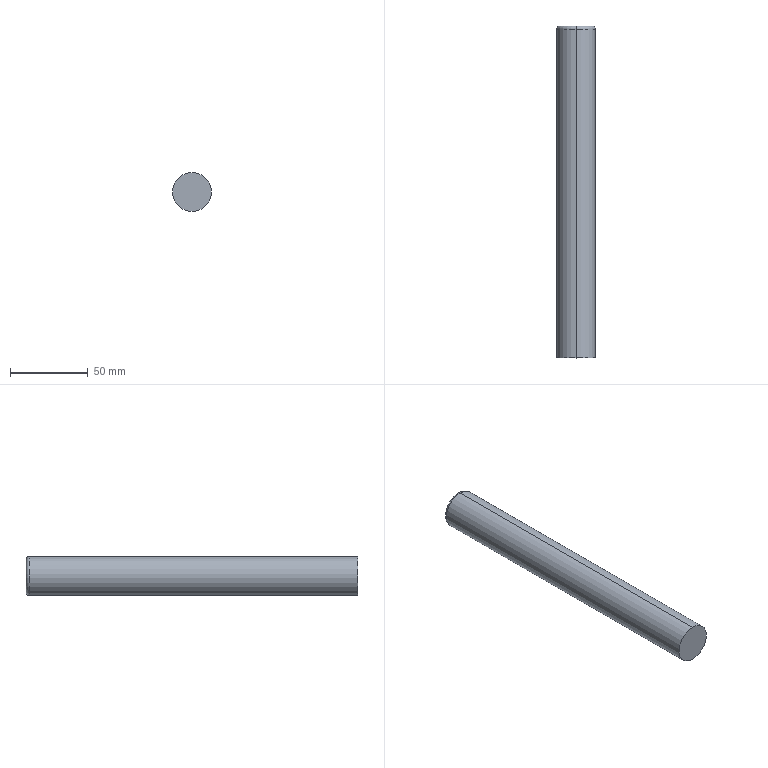Part | SolidWorks | features Extrusion 1, Fillet 1 | 1 solid | 6 faces | box 25 x 213.5 x 25 mm | volume 104737 mm3 | torus 2 | cylinder 2 | plane 2 | commonest cylinder face diameters 25 x2
STEP:
#1=CARTESIAN_POINT('',(0.,211.5,-12.5));
#2=VERTEX_POINT('',#1);
#3=CARTESIAN_POINT('',(0.,211.5,12.5));
#4=VERTEX_POINT('',#3);
#5=CARTESIAN_POINT('',(0.,211.5,0.));
#6=DIRECTION('',(0.,-1.,0.));
#7=DIRECTION('',(0.,0.,1.));
#8=AXIS2_PLACEMENT_3D('',#5,#6,#7);
#9=CIRCLE('',#8,12.5);
#10=EDGE_CURVE('',#2,#4,#9,.T.);
#11=ORIENTED_EDGE('',*,*,#10,.F.);
#12=CARTESIAN_POINT('',(0.,213.5,-10.5));
#13=VERTEX_POINT('',#12);
#14=CARTESIAN_POINT('',(0.,211.5,-10.5));
#15=DIRECTION('',(1.,0.,0.));
#16=DIRECTION('',(0.,0.,-1.));
#17=AXIS2_PLACEMENT_3D('',#14,#15,#16);
#18=CIRCLE('',#17,2.);
#19=EDGE_CURVE('',#2,#13,#18,.T.);
#20=ORIENTED_EDGE('',*,*,#19,.T.);
#21=CARTESIAN_POINT('',(0.,213.5,10.5));
#22=VERTEX_POINT('',#21);
#23=CARTESIAN_POINT('',(0.,213.5,0.));
#24=DIRECTION('',(0.,1.,0.));
#25=DIRECTION('',(0.,0.,1.));
#26=AXIS2_PLACEMENT_3D('',#23,#24,#25);
#27=CIRCLE('',#26,10.5);
#28=EDGE_CURVE('',#22,#13,#27,.T.);
#29=ORIENTED_EDGE('',*,*,#28,.F.);
#30=CARTESIAN_POINT('',(0.,211.5,10.5));
#31=DIRECTION('',(-1.,0.,0.));
#32=DIRECTION('',(0.,0.,1.));
#33=AXIS2_PLACEMENT_3D('',#30,#31,#32);
#34=CIRCLE('',#33,2.);
#35=EDGE_CURVE('',#4,#22,#34,.T.);
#36=ORIENTED_EDGE('',*,*,#35,.F.);
#37=EDGE_LOOP('',(#11,#20,#29,#36));
#38=FACE_OUTER_BOUND('',#37,.T.);
#39=CARTESIAN_POINT('',(0.,211.5,0.));
#40=DIRECTION('',(0.,1.,0.));
#41=DIRECTION('',(0.,0.,1.));
#42=AXIS2_PLACEMENT_3D('',#39,#40,#41);
#43=TOROIDAL_SURFACE('',#42,10.5,2.);
#44=ADVANCED_FACE('',(#38),#43,.T.);
#45=ORIENTED_EDGE('',*,*,#10,.T.);
#46=CARTESIAN_POINT('',(0.,0.,12.5));
#47=VERTEX_POINT('',#46);
#48=CARTESIAN_POINT('',(0.,213.5,12.5));
#49=DIRECTION('',(0.,-1.,0.));
#50=VECTOR('',#49,1000.);
#51=LINE('',#48,#50);
#52=EDGE_CURVE('',#4,#47,#51,.T.);
#53=ORIENTED_EDGE('',*,*,#52,.T.);
#54=CARTESIAN_POINT('',(0.,0.,-12.5));
#55=VERTEX_POINT('',#54);
#56=CARTESIAN_POINT('',(0.,0.,0.));
#57=DIRECTION('',(0.,1.,0.));
#58=DIRECTION('',(0.,0.,1.));
#59=AXIS2_PLACEMENT_3D('',#56,#57,#58);
#60=CIRCLE('',#59,12.5);
#61=EDGE_CURVE('',#47,#55,#60,.T.);
#62=ORIENTED_EDGE('',*,*,#61,.T.);
#63=CARTESIAN_POINT('',(0.,213.5,-12.5));
#64=DIRECTION('',(0.,-1.,0.));
#65=VECTOR('',#64,1000.);
#66=LINE('',#63,#65);
#67=EDGE_CURVE('',#2,#55,#66,.T.);
#68=ORIENTED_EDGE('',*,*,#67,.F.);
#69=EDGE_LOOP('',(#45,#53,#62,#68));
#70=FACE_OUTER_BOUND('',#69,.T.);
#71=CARTESIAN_POINT('',(0.,213.5,0.));
#72=DIRECTION('',(0.,-1.,0.));
#73=DIRECTION('',(0.,0.,-1.));
#74=AXIS2_PLACEMENT_3D('',#71,#72,#73);
#75=CYLINDRICAL_SURFACE('',#74,12.5);
#76=ADVANCED_FACE('',(#70),#75,.T.);
#77=ORIENTED_EDGE('',*,*,#52,.F.);
#78=CARTESIAN_POINT('',(0.,211.5,0.));
#79=DIRECTION('',(0.,-1.,0.));
#80=DIRECTION('',(0.,0.,1.));
#81=AXIS2_PLACEMENT_3D('',#78,#79,#80);
#82=CIRCLE('',#81,12.5);
#83=EDGE_CURVE('',#4,#2,#82,.T.);
#84=ORIENTED_EDGE('',*,*,#83,.T.);
#85=ORIENTED_EDGE('',*,*,#67,.T.);
#86=CARTESIAN_POINT('',(0.,0.,0.));
#87=DIRECTION('',(0.,1.,0.));
#88=DIRECTION('',(0.,0.,1.));
#89=AXIS2_PLACEMENT_3D('',#86,#87,#88);
#90=CIRCLE('',#89,12.5);
#91=EDGE_CURVE('',#55,#47,#90,.T.);
#92=ORIENTED_EDGE('',*,*,#91,.T.);
#93=EDGE_LOOP('',(#77,#84,#85,#92));
#94=FACE_OUTER_BOUND('',#93,.T.);
#95=CARTESIAN_POINT('',(0.,213.5,0.));
#96=DIRECTION('',(0.,-1.,0.));
#97=DIRECTION('',(0.,0.,-1.));
#98=AXIS2_PLACEMENT_3D('',#95,#96,#97);
#99=CYLINDRICAL_SURFACE('',#98,12.5);
#100=ADVANCED_FACE('',(#94),#99,.T.);
#101=ORIENTED_EDGE('',*,*,#28,.T.);
#102=CARTESIAN_POINT('',(0.,213.5,0.));
#103=DIRECTION('',(0.,1.,0.));
#104=DIRECTION('',(0.,0.,1.));
#105=AXIS2_PLACEMENT_3D('',#102,#103,#104);
#106=CIRCLE('',#105,10.5);
#107=EDGE_CURVE('',#13,#22,#106,.T.);
#108=ORIENTED_EDGE('',*,*,#107,.T.);
#109=EDGE_LOOP('',(#101,#108));
#110=FACE_OUTER_BOUND('',#109,.T.);
#111=CARTESIAN_POINT('',(0.,213.5,0.));
#112=DIRECTION('',(0.,1.,0.));
#113=DIRECTION('',(0.,0.,1.));
#114=AXIS2_PLACEMENT_3D('',#111,#112,#113);
#115=PLANE('',#114);
#116=ADVANCED_FACE('',(#110),#115,.T.);
#117=ORIENTED_EDGE('',*,*,#91,.F.);
#118=ORIENTED_EDGE('',*,*,#61,.F.);
#119=EDGE_LOOP('',(#117,#118));
#120=FACE_OUTER_BOUND('',#119,.T.);
#121=CARTESIAN_POINT('',(0.,0.,0.));
#122=DIRECTION('',(0.,1.,0.));
#123=DIRECTION('',(0.,0.,1.));
#124=AXIS2_PLACEMENT_3D('',#121,#122,#123);
#125=PLANE('',#124);
#126=ADVANCED_FACE('',(#120),#125,.F.);
#127=ORIENTED_EDGE('',*,*,#19,.F.);
#128=ORIENTED_EDGE('',*,*,#83,.F.);
#129=ORIENTED_EDGE('',*,*,#35,.T.);
#130=ORIENTED_EDGE('',*,*,#107,.F.);
#131=EDGE_LOOP('',(#127,#128,#129,#130));
#132=FACE_OUTER_BOUND('',#131,.T.);
#133=CARTESIAN_POINT('',(0.,211.5,0.));
#134=DIRECTION('',(0.,1.,0.));
#135=DIRECTION('',(0.,0.,1.));
#136=AXIS2_PLACEMENT_3D('',#133,#134,#135);
#137=TOROIDAL_SURFACE('',#136,10.5,2.);
#138=ADVANCED_FACE('',(#132),#137,.T.);
#139=CLOSED_SHELL('',(#44,#76,#100,#116,#126,#138));
#140=MANIFOLD_SOLID_BREP('',#139);
#141=CARTESIAN_POINT('',(0.,0.,0.));
#142=DIRECTION('',(0.,0.,1.));
#143=DIRECTION('',(1.,0.,0.));
#144=AXIS2_PLACEMENT_3D('',#141,#142,#143);
#145=(LENGTH_UNIT()NAMED_UNIT(*)SI_UNIT(.MILLI.,.METRE.));
#146=UNCERTAINTY_MEASURE_WITH_UNIT(LENGTH_MEASURE(0.00001),#145,'','');
#147=(NAMED_UNIT(*)PLANE_ANGLE_UNIT()SI_UNIT($,.RADIAN.));
#148=(NAMED_UNIT(*)SI_UNIT($,.STERADIAN.)SOLID_ANGLE_UNIT());
#149=(GEOMETRIC_REPRESENTATION_CONTEXT(3)GLOBAL_UNCERTAINTY_ASSIGNED_CONTEXT((#146))GLOBAL_UNIT_ASSIGNED_CONTEXT((#145,#147,#148))REPRESENTATION_CONTEXT('',''));
#150=ADVANCED_BREP_SHAPE_REPRESENTATION('',(#140,#144),#149);